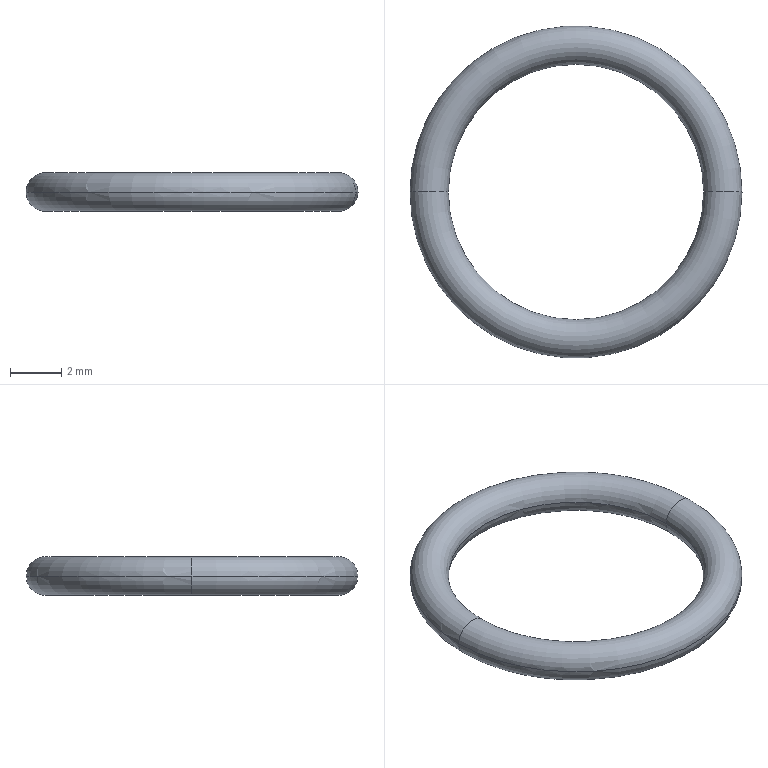Part | STEP file | SOLID | 1 solid | 4 faces | box 13 x 13 x 1.5 mm | volume 63.844 mm3 | torus 4
STEP:
#1=CARTESIAN_POINT('',(0.,0.,0.));
#2=DIRECTION('',(0.,0.,1.));
#3=DIRECTION('',(1.,0.,0.));
#4=AXIS2_PLACEMENT_3D('',#1,#2,#3);
#5=CARTESIAN_POINT('',(-11.5,0.,0.));
#6=VERTEX_POINT('',#5);
#7=CARTESIAN_POINT('',(1.5,0.,0.));
#8=VERTEX_POINT('',#7);
#9=CARTESIAN_POINT('',(-5.,0.,0.));
#10=DIRECTION('',(0.,0.,1.));
#11=DIRECTION('',(1.,0.,0.));
#12=AXIS2_PLACEMENT_3D('',#9,#10,#11);
#13=CIRCLE('',#12,6.5);
#14=CARTESIAN_POINT('',(-5.,0.,0.));
#15=DIRECTION('',(0.,0.,1.));
#16=DIRECTION('',(1.,0.,0.));
#17=AXIS2_PLACEMENT_3D('',#14,#15,#16);
#18=TOROIDAL_SURFACE('',#17,5.75,0.75);
#19=CARTESIAN_POINT('',(0.,6.283));
#20=DIRECTION('',(1.,0.));
#21=VECTOR('',#20,1.);
#22=LINE('',#19,#21);
#23=(GEOMETRIC_REPRESENTATION_CONTEXT(2)PARAMETRIC_REPRESENTATION_CONTEXT()REPRESENTATION_CONTEXT('',''));
#24=DEFINITIONAL_REPRESENTATION('',(#22),#23);
#25=PCURVE('',#18,#24);
#26=CARTESIAN_POINT('',(-5.,0.,0.));
#27=DIRECTION('',(0.,0.,1.));
#28=DIRECTION('',(1.,0.,0.));
#29=AXIS2_PLACEMENT_3D('',#26,#27,#28);
#30=TOROIDAL_SURFACE('',#29,5.75,0.75);
#31=CARTESIAN_POINT('',(0.,0.));
#32=DIRECTION('',(1.,0.));
#33=VECTOR('',#32,1.);
#34=LINE('',#31,#33);
#35=(GEOMETRIC_REPRESENTATION_CONTEXT(2)PARAMETRIC_REPRESENTATION_CONTEXT()REPRESENTATION_CONTEXT('',''));
#36=DEFINITIONAL_REPRESENTATION('',(#34),#35);
#37=PCURVE('',#30,#36);
#38=SURFACE_CURVE('',#13,(#25,#37),.PCURVE_S1.);
#39=EDGE_CURVE('',#6,#8,#38,.T.);
#40=ORIENTED_EDGE('',*,*,#39,.F.);
#41=CARTESIAN_POINT('',(-10.,0.,0.));
#42=VERTEX_POINT('',#41);
#43=CARTESIAN_POINT('',(-10.75,0.,0.));
#44=DIRECTION('',(0.,1.,0.));
#45=DIRECTION('',(-1.,0.,0.));
#46=AXIS2_PLACEMENT_3D('',#43,#44,#45);
#47=CIRCLE('',#46,0.75);
#48=CARTESIAN_POINT('',(3.142,0.));
#49=DIRECTION('',(0.,1.));
#50=VECTOR('',#49,1.);
#51=LINE('',#48,#50);
#52=(GEOMETRIC_REPRESENTATION_CONTEXT(2)PARAMETRIC_REPRESENTATION_CONTEXT()REPRESENTATION_CONTEXT('',''));
#53=DEFINITIONAL_REPRESENTATION('',(#51),#52);
#54=PCURVE('',#18,#53);
#55=CARTESIAN_POINT('',(-5.,0.,0.));
#56=DIRECTION('',(0.,0.,1.));
#57=DIRECTION('',(1.,0.,0.));
#58=AXIS2_PLACEMENT_3D('',#55,#56,#57);
#59=TOROIDAL_SURFACE('',#58,5.75,0.75);
#60=CARTESIAN_POINT('',(3.142,0.));
#61=DIRECTION('',(0.,1.));
#62=VECTOR('',#61,1.);
#63=LINE('',#60,#62);
#64=(GEOMETRIC_REPRESENTATION_CONTEXT(2)PARAMETRIC_REPRESENTATION_CONTEXT()REPRESENTATION_CONTEXT('',''));
#65=DEFINITIONAL_REPRESENTATION('',(#63),#64);
#66=PCURVE('',#59,#65);
#67=SURFACE_CURVE('',#47,(#54,#66),.PCURVE_S1.);
#68=EDGE_CURVE('',#42,#6,#67,.T.);
#69=ORIENTED_EDGE('',*,*,#68,.F.);
#70=CARTESIAN_POINT('',(0.,0.,0.));
#71=VERTEX_POINT('',#70);
#72=CARTESIAN_POINT('',(-5.,0.,0.));
#73=DIRECTION('',(0.,0.,1.));
#74=DIRECTION('',(1.,0.,0.));
#75=AXIS2_PLACEMENT_3D('',#72,#73,#74);
#76=CIRCLE('',#75,5.);
#77=CARTESIAN_POINT('',(0.,3.142));
#78=DIRECTION('',(1.,0.));
#79=VECTOR('',#78,1.);
#80=LINE('',#77,#79);
#81=(GEOMETRIC_REPRESENTATION_CONTEXT(2)PARAMETRIC_REPRESENTATION_CONTEXT()REPRESENTATION_CONTEXT('',''));
#82=DEFINITIONAL_REPRESENTATION('',(#80),#81);
#83=PCURVE('',#18,#82);
#84=CARTESIAN_POINT('',(0.,3.142));
#85=DIRECTION('',(1.,0.));
#86=VECTOR('',#85,1.);
#87=LINE('',#84,#86);
#88=(GEOMETRIC_REPRESENTATION_CONTEXT(2)PARAMETRIC_REPRESENTATION_CONTEXT()REPRESENTATION_CONTEXT('',''));
#89=DEFINITIONAL_REPRESENTATION('',(#87),#88);
#90=PCURVE('',#30,#89);
#91=SURFACE_CURVE('',#76,(#83,#90),.PCURVE_S1.);
#92=EDGE_CURVE('',#42,#71,#91,.T.);
#93=ORIENTED_EDGE('',*,*,#92,.T.);
#94=CARTESIAN_POINT('',(0.75,0.,0.));
#95=DIRECTION('',(0.,-1.,0.));
#96=DIRECTION('',(0.,0.,-1.));
#97=AXIS2_PLACEMENT_3D('',#94,#95,#96);
#98=CIRCLE('',#97,0.75);
#99=CARTESIAN_POINT('',(6.283,-1.571));
#100=DIRECTION('',(0.,1.));
#101=VECTOR('',#100,1.);
#102=LINE('',#99,#101);
#103=(GEOMETRIC_REPRESENTATION_CONTEXT(2)PARAMETRIC_REPRESENTATION_CONTEXT()REPRESENTATION_CONTEXT('',''));
#104=DEFINITIONAL_REPRESENTATION('',(#102),#103);
#105=PCURVE('',#18,#104);
#106=CARTESIAN_POINT('',(0.,-1.571));
#107=DIRECTION('',(0.,1.));
#108=VECTOR('',#107,1.);
#109=LINE('',#106,#108);
#110=(GEOMETRIC_REPRESENTATION_CONTEXT(2)PARAMETRIC_REPRESENTATION_CONTEXT()REPRESENTATION_CONTEXT('',''));
#111=DEFINITIONAL_REPRESENTATION('',(#109),#110);
#112=PCURVE('',#59,#111);
#113=SURFACE_CURVE('',#98,(#105,#112),.PCURVE_S1.);
#114=EDGE_CURVE('',#71,#8,#113,.T.);
#115=ORIENTED_EDGE('',*,*,#114,.T.);
#116=EDGE_LOOP('',(#40,#69,#93,#115));
#117=FACE_BOUND('',#116,.T.);
#118=ADVANCED_FACE('',(#117),#18,.T.);
#119=CARTESIAN_POINT('',(-5.,0.,0.));
#120=DIRECTION('',(0.,0.,1.));
#121=DIRECTION('',(1.,0.,0.));
#122=AXIS2_PLACEMENT_3D('',#119,#120,#121);
#123=CIRCLE('',#122,6.5);
#124=CARTESIAN_POINT('',(0.,6.283));
#125=DIRECTION('',(1.,0.));
#126=VECTOR('',#125,1.);
#127=LINE('',#124,#126);
#128=(GEOMETRIC_REPRESENTATION_CONTEXT(2)PARAMETRIC_REPRESENTATION_CONTEXT()REPRESENTATION_CONTEXT('',''));
#129=DEFINITIONAL_REPRESENTATION('',(#127),#128);
#130=PCURVE('',#59,#129);
#131=CARTESIAN_POINT('',(-5.,0.,0.));
#132=DIRECTION('',(0.,0.,1.));
#133=DIRECTION('',(1.,0.,0.));
#134=AXIS2_PLACEMENT_3D('',#131,#132,#133);
#135=TOROIDAL_SURFACE('',#134,5.75,0.75);
#136=CARTESIAN_POINT('',(0.,0.));
#137=DIRECTION('',(1.,0.));
#138=VECTOR('',#137,1.);
#139=LINE('',#136,#138);
#140=(GEOMETRIC_REPRESENTATION_CONTEXT(2)PARAMETRIC_REPRESENTATION_CONTEXT()REPRESENTATION_CONTEXT('',''));
#141=DEFINITIONAL_REPRESENTATION('',(#139),#140);
#142=PCURVE('',#135,#141);
#143=SURFACE_CURVE('',#123,(#130,#142),.PCURVE_S1.);
#144=EDGE_CURVE('',#8,#6,#143,.T.);
#145=ORIENTED_EDGE('',*,*,#144,.F.);
#146=ORIENTED_EDGE('',*,*,#114,.F.);
#147=CARTESIAN_POINT('',(-5.,0.,0.));
#148=DIRECTION('',(0.,0.,1.));
#149=DIRECTION('',(1.,0.,0.));
#150=AXIS2_PLACEMENT_3D('',#147,#148,#149);
#151=CIRCLE('',#150,5.);
#152=CARTESIAN_POINT('',(0.,3.142));
#153=DIRECTION('',(1.,0.));
#154=VECTOR('',#153,1.);
#155=LINE('',#152,#154);
#156=(GEOMETRIC_REPRESENTATION_CONTEXT(2)PARAMETRIC_REPRESENTATION_CONTEXT()REPRESENTATION_CONTEXT('',''));
#157=DEFINITIONAL_REPRESENTATION('',(#155),#156);
#158=PCURVE('',#59,#157);
#159=CARTESIAN_POINT('',(0.,3.142));
#160=DIRECTION('',(1.,0.));
#161=VECTOR('',#160,1.);
#162=LINE('',#159,#161);
#163=(GEOMETRIC_REPRESENTATION_CONTEXT(2)PARAMETRIC_REPRESENTATION_CONTEXT()REPRESENTATION_CONTEXT('',''));
#164=DEFINITIONAL_REPRESENTATION('',(#162),#163);
#165=PCURVE('',#135,#164);
#166=SURFACE_CURVE('',#151,(#158,#165),.PCURVE_S1.);
#167=EDGE_CURVE('',#71,#42,#166,.T.);
#168=ORIENTED_EDGE('',*,*,#167,.T.);
#169=ORIENTED_EDGE('',*,*,#68,.T.);
#170=EDGE_LOOP('',(#145,#146,#168,#169));
#171=FACE_BOUND('',#170,.T.);
#172=ADVANCED_FACE('',(#171),#59,.T.);
#173=CARTESIAN_POINT('',(0.75,0.,0.));
#174=DIRECTION('',(0.,-1.,0.));
#175=DIRECTION('',(0.,0.,-1.));
#176=AXIS2_PLACEMENT_3D('',#173,#174,#175);
#177=CIRCLE('',#176,0.75);
#178=CARTESIAN_POINT('',(0.,-1.571));
#179=DIRECTION('',(0.,1.));
#180=VECTOR('',#179,1.);
#181=LINE('',#178,#180);
#182=(GEOMETRIC_REPRESENTATION_CONTEXT(2)PARAMETRIC_REPRESENTATION_CONTEXT()REPRESENTATION_CONTEXT('',''));
#183=DEFINITIONAL_REPRESENTATION('',(#181),#182);
#184=PCURVE('',#135,#183);
#185=CARTESIAN_POINT('',(6.283,-1.571));
#186=DIRECTION('',(0.,1.));
#187=VECTOR('',#186,1.);
#188=LINE('',#185,#187);
#189=(GEOMETRIC_REPRESENTATION_CONTEXT(2)PARAMETRIC_REPRESENTATION_CONTEXT()REPRESENTATION_CONTEXT('',''));
#190=DEFINITIONAL_REPRESENTATION('',(#188),#189);
#191=PCURVE('',#30,#190);
#192=SURFACE_CURVE('',#177,(#184,#191),.PCURVE_S1.);
#193=EDGE_CURVE('',#8,#71,#192,.T.);
#194=ORIENTED_EDGE('',*,*,#193,.F.);
#195=ORIENTED_EDGE('',*,*,#144,.T.);
#196=CARTESIAN_POINT('',(-10.75,0.,0.));
#197=DIRECTION('',(0.,1.,0.));
#198=DIRECTION('',(-1.,0.,0.));
#199=AXIS2_PLACEMENT_3D('',#196,#197,#198);
#200=CIRCLE('',#199,0.75);
#201=CARTESIAN_POINT('',(3.142,0.));
#202=DIRECTION('',(0.,1.));
#203=VECTOR('',#202,1.);
#204=LINE('',#201,#203);
#205=(GEOMETRIC_REPRESENTATION_CONTEXT(2)PARAMETRIC_REPRESENTATION_CONTEXT()REPRESENTATION_CONTEXT('',''));
#206=DEFINITIONAL_REPRESENTATION('',(#204),#205);
#207=PCURVE('',#135,#206);
#208=CARTESIAN_POINT('',(3.142,0.));
#209=DIRECTION('',(0.,1.));
#210=VECTOR('',#209,1.);
#211=LINE('',#208,#210);
#212=(GEOMETRIC_REPRESENTATION_CONTEXT(2)PARAMETRIC_REPRESENTATION_CONTEXT()REPRESENTATION_CONTEXT('',''));
#213=DEFINITIONAL_REPRESENTATION('',(#211),#212);
#214=PCURVE('',#30,#213);
#215=SURFACE_CURVE('',#200,(#207,#214),.PCURVE_S1.);
#216=EDGE_CURVE('',#6,#42,#215,.T.);
#217=ORIENTED_EDGE('',*,*,#216,.T.);
#218=ORIENTED_EDGE('',*,*,#167,.F.);
#219=EDGE_LOOP('',(#194,#195,#217,#218));
#220=FACE_BOUND('',#219,.T.);
#221=ADVANCED_FACE('',(#220),#135,.T.);
#222=ORIENTED_EDGE('',*,*,#216,.F.);
#223=ORIENTED_EDGE('',*,*,#39,.T.);
#224=ORIENTED_EDGE('',*,*,#193,.T.);
#225=ORIENTED_EDGE('',*,*,#92,.F.);
#226=EDGE_LOOP('',(#222,#223,#224,#225));
#227=FACE_BOUND('',#226,.T.);
#228=ADVANCED_FACE('',(#227),#30,.T.);
#229=CLOSED_SHELL('',(#118,#172,#221,#228));
#230=MANIFOLD_SOLID_BREP('',#229);
#231=(LENGTH_UNIT()NAMED_UNIT(*)SI_UNIT(.MILLI.,.METRE.));
#232=UNCERTAINTY_MEASURE_WITH_UNIT(LENGTH_MEASURE(0.0000001),#231,'','');
#233=(NAMED_UNIT(*)PLANE_ANGLE_UNIT()SI_UNIT($,.RADIAN.));
#234=(NAMED_UNIT(*)SI_UNIT($,.STERADIAN.)SOLID_ANGLE_UNIT());
#235=(GEOMETRIC_REPRESENTATION_CONTEXT(3)GLOBAL_UNCERTAINTY_ASSIGNED_CONTEXT((#232))GLOBAL_UNIT_ASSIGNED_CONTEXT((#231,#233,#234))REPRESENTATION_CONTEXT('',''));
#236=ADVANCED_BREP_SHAPE_REPRESENTATION('',(#4,#230),#235);